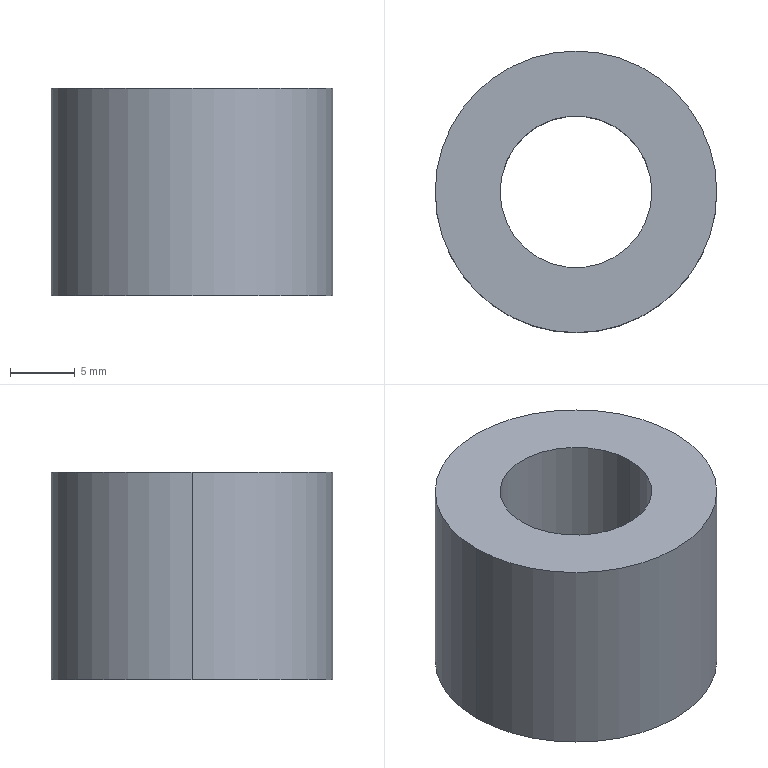Part | SolidWorks | features Extrusion 1 | 1 solid | 6 faces | box 21.7 x 21.7 x 16 mm | volume 4197 mm3 | cylinder 4 | plane 2 | commonest cylinder face diameters 11.7 x2 21.7 x2
STEP:
#1=CARTESIAN_POINT('',(-5.85,0.,16.));
#2=VERTEX_POINT('',#1);
#3=CARTESIAN_POINT('',(5.85,0.,16.));
#4=VERTEX_POINT('',#3);
#5=CARTESIAN_POINT('',(0.,0.,16.));
#6=DIRECTION('',(0.,0.,1.));
#7=DIRECTION('',(1.,0.,0.));
#8=AXIS2_PLACEMENT_3D('',#5,#6,#7);
#9=CIRCLE('',#8,5.85);
#10=EDGE_CURVE('',#2,#4,#9,.T.);
#11=ORIENTED_EDGE('',*,*,#10,.T.);
#12=CARTESIAN_POINT('',(5.85,0.,0.));
#13=VERTEX_POINT('',#12);
#14=CARTESIAN_POINT('',(5.85,0.,16.));
#15=DIRECTION('',(0.,0.,-1.));
#16=VECTOR('',#15,1000.);
#17=LINE('',#14,#16);
#18=EDGE_CURVE('',#4,#13,#17,.T.);
#19=ORIENTED_EDGE('',*,*,#18,.T.);
#20=CARTESIAN_POINT('',(-5.85,0.,0.));
#21=VERTEX_POINT('',#20);
#22=CARTESIAN_POINT('',(0.,0.,0.));
#23=DIRECTION('',(0.,0.,1.));
#24=DIRECTION('',(1.,0.,0.));
#25=AXIS2_PLACEMENT_3D('',#22,#23,#24);
#26=CIRCLE('',#25,5.85);
#27=EDGE_CURVE('',#21,#13,#26,.T.);
#28=ORIENTED_EDGE('',*,*,#27,.F.);
#29=CARTESIAN_POINT('',(-5.85,0.,16.));
#30=DIRECTION('',(0.,0.,-1.));
#31=VECTOR('',#30,1000.);
#32=LINE('',#29,#31);
#33=EDGE_CURVE('',#2,#21,#32,.T.);
#34=ORIENTED_EDGE('',*,*,#33,.F.);
#35=EDGE_LOOP('',(#11,#19,#28,#34));
#36=FACE_OUTER_BOUND('',#35,.T.);
#37=CARTESIAN_POINT('',(0.,0.,16.));
#38=DIRECTION('',(0.,0.,-1.));
#39=DIRECTION('',(-1.,0.,0.));
#40=AXIS2_PLACEMENT_3D('',#37,#38,#39);
#41=CYLINDRICAL_SURFACE('',#40,5.85);
#42=ADVANCED_FACE('',(#36),#41,.F.);
#43=CARTESIAN_POINT('',(10.85,0.,16.));
#44=VERTEX_POINT('',#43);
#45=CARTESIAN_POINT('',(-10.85,0.,16.));
#46=VERTEX_POINT('',#45);
#47=CARTESIAN_POINT('',(0.,0.,16.));
#48=DIRECTION('',(0.,0.,1.));
#49=DIRECTION('',(1.,0.,0.));
#50=AXIS2_PLACEMENT_3D('',#47,#48,#49);
#51=CIRCLE('',#50,10.85);
#52=EDGE_CURVE('',#44,#46,#51,.T.);
#53=ORIENTED_EDGE('',*,*,#52,.F.);
#54=CARTESIAN_POINT('',(10.85,0.,0.));
#55=VERTEX_POINT('',#54);
#56=CARTESIAN_POINT('',(10.85,0.,16.));
#57=DIRECTION('',(0.,0.,-1.));
#58=VECTOR('',#57,1000.);
#59=LINE('',#56,#58);
#60=EDGE_CURVE('',#44,#55,#59,.T.);
#61=ORIENTED_EDGE('',*,*,#60,.T.);
#62=CARTESIAN_POINT('',(-10.85,0.,0.));
#63=VERTEX_POINT('',#62);
#64=CARTESIAN_POINT('',(0.,0.,0.));
#65=DIRECTION('',(0.,0.,1.));
#66=DIRECTION('',(1.,0.,0.));
#67=AXIS2_PLACEMENT_3D('',#64,#65,#66);
#68=CIRCLE('',#67,10.85);
#69=EDGE_CURVE('',#55,#63,#68,.T.);
#70=ORIENTED_EDGE('',*,*,#69,.T.);
#71=CARTESIAN_POINT('',(-10.85,0.,16.));
#72=DIRECTION('',(0.,0.,-1.));
#73=VECTOR('',#72,1000.);
#74=LINE('',#71,#73);
#75=EDGE_CURVE('',#46,#63,#74,.T.);
#76=ORIENTED_EDGE('',*,*,#75,.F.);
#77=EDGE_LOOP('',(#53,#61,#70,#76));
#78=FACE_OUTER_BOUND('',#77,.T.);
#79=CARTESIAN_POINT('',(0.,0.,16.));
#80=DIRECTION('',(0.,0.,-1.));
#81=DIRECTION('',(-1.,0.,0.));
#82=AXIS2_PLACEMENT_3D('',#79,#80,#81);
#83=CYLINDRICAL_SURFACE('',#82,10.85);
#84=ADVANCED_FACE('',(#78),#83,.T.);
#85=CARTESIAN_POINT('',(0.,0.,16.));
#86=DIRECTION('',(0.,0.,1.));
#87=DIRECTION('',(1.,0.,0.));
#88=AXIS2_PLACEMENT_3D('',#85,#86,#87);
#89=CIRCLE('',#88,10.85);
#90=EDGE_CURVE('',#46,#44,#89,.T.);
#91=ORIENTED_EDGE('',*,*,#90,.T.);
#92=ORIENTED_EDGE('',*,*,#52,.T.);
#93=EDGE_LOOP('',(#91,#92));
#94=FACE_OUTER_BOUND('',#93,.T.);
#95=ORIENTED_EDGE('',*,*,#10,.F.);
#96=CARTESIAN_POINT('',(0.,0.,16.));
#97=DIRECTION('',(0.,0.,1.));
#98=DIRECTION('',(1.,0.,0.));
#99=AXIS2_PLACEMENT_3D('',#96,#97,#98);
#100=CIRCLE('',#99,5.85);
#101=EDGE_CURVE('',#4,#2,#100,.T.);
#102=ORIENTED_EDGE('',*,*,#101,.F.);
#103=EDGE_LOOP('',(#95,#102));
#104=FACE_BOUND('',#103,.T.);
#105=CARTESIAN_POINT('',(0.,0.,16.));
#106=DIRECTION('',(0.,0.,1.));
#107=DIRECTION('',(1.,0.,0.));
#108=AXIS2_PLACEMENT_3D('',#105,#106,#107);
#109=PLANE('',#108);
#110=ADVANCED_FACE('',(#94,#104),#109,.T.);
#111=CARTESIAN_POINT('',(0.,0.,0.));
#112=DIRECTION('',(0.,0.,1.));
#113=DIRECTION('',(1.,0.,0.));
#114=AXIS2_PLACEMENT_3D('',#111,#112,#113);
#115=CIRCLE('',#114,10.85);
#116=EDGE_CURVE('',#63,#55,#115,.T.);
#117=ORIENTED_EDGE('',*,*,#116,.F.);
#118=ORIENTED_EDGE('',*,*,#69,.F.);
#119=EDGE_LOOP('',(#117,#118));
#120=FACE_OUTER_BOUND('',#119,.T.);
#121=ORIENTED_EDGE('',*,*,#27,.T.);
#122=CARTESIAN_POINT('',(0.,0.,0.));
#123=DIRECTION('',(0.,0.,1.));
#124=DIRECTION('',(1.,0.,0.));
#125=AXIS2_PLACEMENT_3D('',#122,#123,#124);
#126=CIRCLE('',#125,5.85);
#127=EDGE_CURVE('',#13,#21,#126,.T.);
#128=ORIENTED_EDGE('',*,*,#127,.T.);
#129=EDGE_LOOP('',(#121,#128));
#130=FACE_BOUND('',#129,.T.);
#131=CARTESIAN_POINT('',(0.,0.,0.));
#132=DIRECTION('',(0.,0.,1.));
#133=DIRECTION('',(1.,0.,0.));
#134=AXIS2_PLACEMENT_3D('',#131,#132,#133);
#135=PLANE('',#134);
#136=ADVANCED_FACE('',(#120,#130),#135,.F.);
#137=ORIENTED_EDGE('',*,*,#60,.F.);
#138=ORIENTED_EDGE('',*,*,#90,.F.);
#139=ORIENTED_EDGE('',*,*,#75,.T.);
#140=ORIENTED_EDGE('',*,*,#116,.T.);
#141=EDGE_LOOP('',(#137,#138,#139,#140));
#142=FACE_OUTER_BOUND('',#141,.T.);
#143=CARTESIAN_POINT('',(0.,0.,16.));
#144=DIRECTION('',(0.,0.,-1.));
#145=DIRECTION('',(-1.,0.,0.));
#146=AXIS2_PLACEMENT_3D('',#143,#144,#145);
#147=CYLINDRICAL_SURFACE('',#146,10.85);
#148=ADVANCED_FACE('',(#142),#147,.T.);
#149=ORIENTED_EDGE('',*,*,#18,.F.);
#150=ORIENTED_EDGE('',*,*,#101,.T.);
#151=ORIENTED_EDGE('',*,*,#33,.T.);
#152=ORIENTED_EDGE('',*,*,#127,.F.);
#153=EDGE_LOOP('',(#149,#150,#151,#152));
#154=FACE_OUTER_BOUND('',#153,.T.);
#155=CARTESIAN_POINT('',(0.,0.,16.));
#156=DIRECTION('',(0.,0.,-1.));
#157=DIRECTION('',(-1.,0.,0.));
#158=AXIS2_PLACEMENT_3D('',#155,#156,#157);
#159=CYLINDRICAL_SURFACE('',#158,5.85);
#160=ADVANCED_FACE('',(#154),#159,.F.);
#161=CLOSED_SHELL('',(#42,#84,#110,#136,#148,#160));
#162=MANIFOLD_SOLID_BREP('',#161);
#163=CARTESIAN_POINT('',(0.,0.,0.));
#164=DIRECTION('',(0.,0.,1.));
#165=DIRECTION('',(1.,0.,0.));
#166=AXIS2_PLACEMENT_3D('',#163,#164,#165);
#167=(LENGTH_UNIT()NAMED_UNIT(*)SI_UNIT(.MILLI.,.METRE.));
#168=UNCERTAINTY_MEASURE_WITH_UNIT(LENGTH_MEASURE(0.00001),#167,'','');
#169=(NAMED_UNIT(*)PLANE_ANGLE_UNIT()SI_UNIT($,.RADIAN.));
#170=(NAMED_UNIT(*)SI_UNIT($,.STERADIAN.)SOLID_ANGLE_UNIT());
#171=(GEOMETRIC_REPRESENTATION_CONTEXT(3)GLOBAL_UNCERTAINTY_ASSIGNED_CONTEXT((#168))GLOBAL_UNIT_ASSIGNED_CONTEXT((#167,#169,#170))REPRESENTATION_CONTEXT('',''));
#172=ADVANCED_BREP_SHAPE_REPRESENTATION('',(#162,#166),#171);